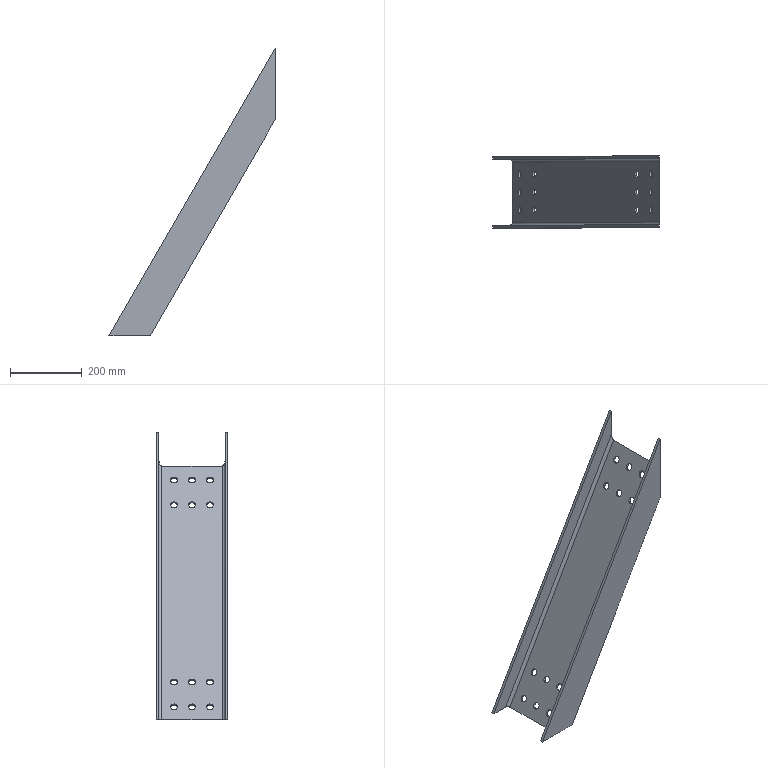Part | STEP file | 粉仓Diagonal Brace梁7_Default<As Machined> | 1 solid | 42 faces | box 462.735 x 200 x 801.481 mm | volume 2141507 mm3 | cylinder 28 | plane 14 | commonest cylinder face diameters 19 x24 16 x4